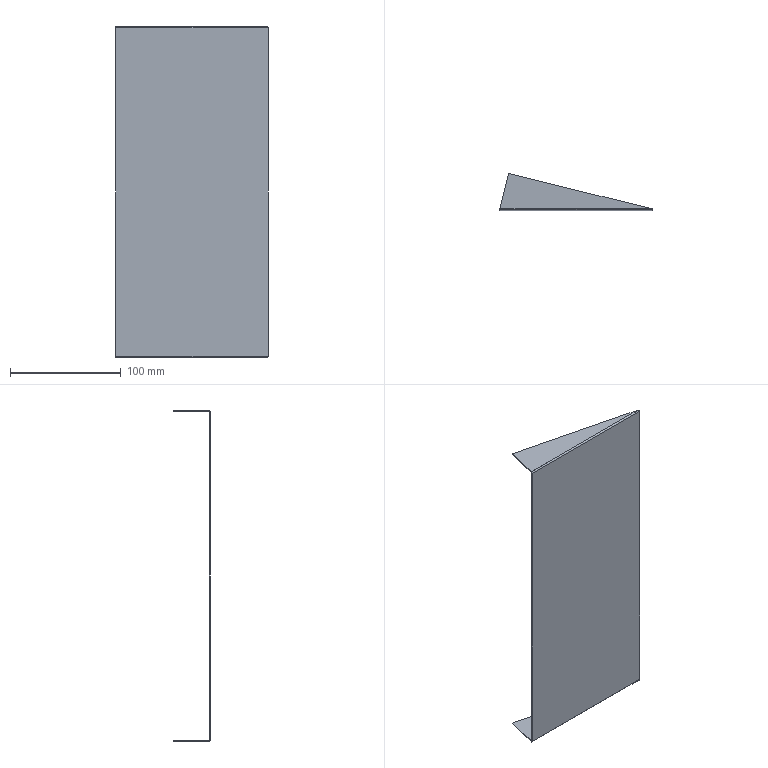Part | SolidWorks | features EdgeFlange 1, FlatPattern 1, MirrorPattern 1, SMBaseFlange 1, SheetMetal 1 | 1 solid | 20 faces | box 137.5 x 33 x 299 mm | volume 45429 mm3 | plane 12 | spline 4 | cylinder 4 | commonest cylinder face diameters 0.4 x2 2.4 x2
STEP:
#1=CARTESIAN_POINT('',(0.,-1.,148.3));
#2=VERTEX_POINT('',#1);
#3=CARTESIAN_POINT('',(-137.5,-1.,148.3));
#4=VERTEX_POINT('',#3);
#5=CARTESIAN_POINT('',(0.,-1.,148.3));
#6=DIRECTION('',(-1.,0.,0.));
#7=VECTOR('',#6,1000.);
#8=LINE('',#5,#7);
#9=EDGE_CURVE('',#2,#4,#8,.T.);
#10=ORIENTED_EDGE('',*,*,#9,.T.);
#11=CARTESIAN_POINT('',(-137.5,-1.,-148.3));
#12=VERTEX_POINT('',#11);
#13=CARTESIAN_POINT('',(-137.5,-1.,149.5));
#14=DIRECTION('',(0.,0.,-1.));
#15=VECTOR('',#14,1000.);
#16=LINE('',#13,#15);
#17=EDGE_CURVE('',#4,#12,#16,.T.);
#18=ORIENTED_EDGE('',*,*,#17,.T.);
#19=CARTESIAN_POINT('',(0.,-1.,-148.3));
#20=VERTEX_POINT('',#19);
#21=CARTESIAN_POINT('',(-137.5,-1.,-148.3));
#22=DIRECTION('',(1.,0.,0.));
#23=VECTOR('',#22,1000.);
#24=LINE('',#21,#23);
#25=EDGE_CURVE('',#12,#20,#24,.T.);
#26=ORIENTED_EDGE('',*,*,#25,.T.);
#27=CARTESIAN_POINT('',(0.,-1.,149.5));
#28=DIRECTION('',(0.,0.,-1.));
#29=VECTOR('',#28,1000.);
#30=LINE('',#27,#29);
#31=EDGE_CURVE('',#2,#20,#30,.T.);
#32=ORIENTED_EDGE('',*,*,#31,.F.);
#33=EDGE_LOOP('',(#10,#18,#26,#32));
#34=FACE_OUTER_BOUND('',#33,.T.);
#35=CARTESIAN_POINT('',(-137.5,-1.,149.5));
#36=DIRECTION('',(0.,1.,0.));
#37=DIRECTION('',(0.,0.,1.));
#38=AXIS2_PLACEMENT_3D('',#35,#36,#37);
#39=PLANE('',#38);
#40=ADVANCED_FACE('',(#34),#39,.F.);
#41=CARTESIAN_POINT('',(-137.5,0.,148.3));
#42=VERTEX_POINT('',#41);
#43=CARTESIAN_POINT('',(-137.5,0.,-148.3));
#44=VERTEX_POINT('',#43);
#45=CARTESIAN_POINT('',(-137.5,0.,149.5));
#46=DIRECTION('',(0.,0.,-1.));
#47=VECTOR('',#46,1000.);
#48=LINE('',#45,#47);
#49=EDGE_CURVE('',#42,#44,#48,.T.);
#50=ORIENTED_EDGE('',*,*,#49,.F.);
#51=CARTESIAN_POINT('',(0.,0.,148.3));
#52=VERTEX_POINT('',#51);
#53=CARTESIAN_POINT('',(0.,0.,148.3));
#54=DIRECTION('',(-1.,0.,0.));
#55=VECTOR('',#54,1000.);
#56=LINE('',#53,#55);
#57=EDGE_CURVE('',#52,#42,#56,.T.);
#58=ORIENTED_EDGE('',*,*,#57,.F.);
#59=CARTESIAN_POINT('',(0.,0.,-148.3));
#60=VERTEX_POINT('',#59);
#61=CARTESIAN_POINT('',(0.,0.,149.5));
#62=DIRECTION('',(0.,0.,-1.));
#63=VECTOR('',#62,1000.);
#64=LINE('',#61,#63);
#65=EDGE_CURVE('',#52,#60,#64,.T.);
#66=ORIENTED_EDGE('',*,*,#65,.T.);
#67=CARTESIAN_POINT('',(-137.5,0.,-148.3));
#68=DIRECTION('',(1.,0.,0.));
#69=VECTOR('',#68,1000.);
#70=LINE('',#67,#69);
#71=EDGE_CURVE('',#44,#60,#70,.T.);
#72=ORIENTED_EDGE('',*,*,#71,.F.);
#73=EDGE_LOOP('',(#50,#58,#66,#72));
#74=FACE_OUTER_BOUND('',#73,.T.);
#75=CARTESIAN_POINT('',(-137.5,0.,149.5));
#76=DIRECTION('',(0.,1.,0.));
#77=DIRECTION('',(0.,0.,1.));
#78=AXIS2_PLACEMENT_3D('',#75,#76,#77);
#79=PLANE('',#78);
#80=ADVANCED_FACE('',(#74),#79,.T.);
#81=ORIENTED_EDGE('',*,*,#65,.F.);
#82=CARTESIAN_POINT('',(0.,0.,148.3));
#83=DIRECTION('',(0.,-1.,0.));
#84=VECTOR('',#83,1000.);
#85=LINE('',#82,#84);
#86=EDGE_CURVE('',#52,#2,#85,.T.);
#87=ORIENTED_EDGE('',*,*,#86,.T.);
#88=ORIENTED_EDGE('',*,*,#31,.T.);
#89=CARTESIAN_POINT('',(0.,0.,-148.3));
#90=DIRECTION('',(0.,-1.,0.));
#91=VECTOR('',#90,1000.);
#92=LINE('',#89,#91);
#93=EDGE_CURVE('',#60,#20,#92,.T.);
#94=ORIENTED_EDGE('',*,*,#93,.F.);
#95=EDGE_LOOP('',(#81,#87,#88,#94));
#96=FACE_OUTER_BOUND('',#95,.T.);
#97=CARTESIAN_POINT('',(0.,0.,149.5));
#98=DIRECTION('',(1.,0.,0.));
#99=DIRECTION('',(0.,0.,-1.));
#100=AXIS2_PLACEMENT_3D('',#97,#98,#99);
#101=PLANE('',#100);
#102=ADVANCED_FACE('',(#96),#101,.T.);
#103=CARTESIAN_POINT('',(-137.5,0.,148.3));
#104=DIRECTION('',(0.,-1.,0.));
#105=VECTOR('',#104,1000.);
#106=LINE('',#103,#105);
#107=EDGE_CURVE('',#42,#4,#106,.T.);
#108=ORIENTED_EDGE('',*,*,#107,.F.);
#109=ORIENTED_EDGE('',*,*,#49,.T.);
#110=CARTESIAN_POINT('',(-137.5,0.,-148.3));
#111=DIRECTION('',(0.,-1.,0.));
#112=VECTOR('',#111,1000.);
#113=LINE('',#110,#112);
#114=EDGE_CURVE('',#44,#12,#113,.T.);
#115=ORIENTED_EDGE('',*,*,#114,.T.);
#116=ORIENTED_EDGE('',*,*,#17,.F.);
#117=EDGE_LOOP('',(#108,#109,#115,#116));
#118=FACE_OUTER_BOUND('',#117,.T.);
#119=CARTESIAN_POINT('',(-137.5,-1.,149.5));
#120=DIRECTION('',(-1.,0.,0.));
#121=DIRECTION('',(0.,0.,1.));
#122=AXIS2_PLACEMENT_3D('',#119,#120,#121);
#123=PLANE('',#122);
#124=ADVANCED_FACE('',(#118),#123,.T.);
#125=CARTESIAN_POINT('',(-0.81,0.2,-148.5));
#126=VERTEX_POINT('',#125);
#127=CARTESIAN_POINT('',(-0.81,0.2,-149.5));
#128=VERTEX_POINT('',#127);
#129=CARTESIAN_POINT('',(-0.81,0.2,-149.5));
#130=DIRECTION('',(0.,0.,-1.));
#131=VECTOR('',#130,1000.);
#132=LINE('',#129,#131);
#133=EDGE_CURVE('',#126,#128,#132,.T.);
#134=ORIENTED_EDGE('',*,*,#133,.F.);
#135=CARTESIAN_POINT('',(0.,0.,-148.3));
#136=CARTESIAN_POINT('',(-0.135,0.,-148.352));
#137=CARTESIAN_POINT('',(-0.27,0.02155,-148.404));
#138=CARTESIAN_POINT('',(-0.54,0.0956,-148.478));
#139=CARTESIAN_POINT('',(-0.675,0.1476,-148.5));
#140=CARTESIAN_POINT('',(-0.81,0.2,-148.5));
#141=B_SPLINE_CURVE_WITH_KNOTS('',3,(#135,#136,#137,#138,#139,#140),.UNSPECIFIED.,.F.,.F.,(4,2,4),(0.,0.5,1.),.UNSPECIFIED.);
#142=EDGE_CURVE('',#60,#126,#141,.T.);
#143=ORIENTED_EDGE('',*,*,#142,.F.);
#144=ORIENTED_EDGE('',*,*,#93,.T.);
#145=CARTESIAN_POINT('',(0.,-1.,-148.3));
#146=CARTESIAN_POINT('',(-0.06814,-1.,-148.459));
#147=CARTESIAN_POINT('',(-0.1341,-0.9695,-148.612));
#148=CARTESIAN_POINT('',(-0.2703,-0.8484,-148.905));
#149=CARTESIAN_POINT('',(-0.3368,-0.7606,-149.036));
#150=CARTESIAN_POINT('',(-0.4727,-0.5372,-149.26));
#151=CARTESIAN_POINT('',(-0.5396,-0.4051,-149.348));
#152=CARTESIAN_POINT('',(-0.675,-0.1141,-149.469));
#153=CARTESIAN_POINT('',(-0.7418,0.04142,-149.5));
#154=CARTESIAN_POINT('',(-0.81,0.2,-149.5));
#155=B_SPLINE_CURVE_WITH_KNOTS('',3,(#145,#146,#147,#148,#149,#150,#151,#152,#153,#154),.UNSPECIFIED.,.F.,.F.,(4,2,2,2,4),(0.,0.0005093,0.001019,0.001528,0.002037),.UNSPECIFIED.);
#156=EDGE_CURVE('',#20,#128,#155,.T.);
#157=ORIENTED_EDGE('',*,*,#156,.T.);
#158=EDGE_LOOP('',(#134,#143,#144,#157));
#159=FACE_OUTER_BOUND('',#158,.T.);
#160=CARTESIAN_POINT('',(0.,-1.01,-148.3));
#161=CARTESIAN_POINT('',(-0.06751,-1.01,-148.458));
#162=CARTESIAN_POINT('',(-0.135,-0.9785,-148.617));
#163=CARTESIAN_POINT('',(-0.27,-0.8573,-148.909));
#164=CARTESIAN_POINT('',(-0.3375,-0.7676,-149.044));
#165=CARTESIAN_POINT('',(-0.4725,-0.5436,-149.268));
#166=CARTESIAN_POINT('',(-0.54,-0.4094,-149.357));
#167=CARTESIAN_POINT('',(-0.675,-0.1167,-149.479));
#168=CARTESIAN_POINT('',(-0.7425,0.04159,-149.51));
#169=CARTESIAN_POINT('',(-0.81,0.2,-149.51));
#170=CARTESIAN_POINT('',(0.,-1.,-148.3));
#171=CARTESIAN_POINT('',(-0.06751,-1.,-148.457));
#172=CARTESIAN_POINT('',(-0.135,-0.9688,-148.614));
#173=CARTESIAN_POINT('',(-0.27,-0.8485,-148.904));
#174=CARTESIAN_POINT('',(-0.3375,-0.7596,-149.037));
#175=CARTESIAN_POINT('',(-0.4725,-0.5375,-149.26));
#176=CARTESIAN_POINT('',(-0.54,-0.4043,-149.349));
#177=CARTESIAN_POINT('',(-0.675,-0.1141,-149.469));
#178=CARTESIAN_POINT('',(-0.7425,0.0429,-149.5));
#179=CARTESIAN_POINT('',(-0.81,0.2,-149.5));
#180=CARTESIAN_POINT('',(0.,0.,-148.3));
#181=CARTESIAN_POINT('',(-0.0675,0.,-148.326));
#182=CARTESIAN_POINT('',(-0.135,0.005205,-148.352));
#183=CARTESIAN_POINT('',(-0.27,0.02524,-148.401));
#184=CARTESIAN_POINT('',(-0.3375,0.04007,-148.423));
#185=CARTESIAN_POINT('',(-0.4725,0.07709,-148.46));
#186=CARTESIAN_POINT('',(-0.54,0.09928,-148.475));
#187=CARTESIAN_POINT('',(-0.675,0.1477,-148.495));
#188=CARTESIAN_POINT('',(-0.7425,0.1738,-148.5));
#189=CARTESIAN_POINT('',(-0.81,0.2,-148.5));
#190=CARTESIAN_POINT('',(0.,0.0101,-148.3));
#191=CARTESIAN_POINT('',(-0.0675,0.0101,-148.325));
#192=CARTESIAN_POINT('',(-0.135,0.01504,-148.35));
#193=CARTESIAN_POINT('',(-0.27,0.03407,-148.396));
#194=CARTESIAN_POINT('',(-0.3375,0.04814,-148.417));
#195=CARTESIAN_POINT('',(-0.4725,0.0833,-148.452));
#196=CARTESIAN_POINT('',(-0.54,0.1044,-148.466));
#197=CARTESIAN_POINT('',(-0.675,0.1503,-148.485));
#198=CARTESIAN_POINT('',(-0.7425,0.1751,-148.49));
#199=CARTESIAN_POINT('',(-0.81,0.2,-148.49));
#200=B_SPLINE_SURFACE_WITH_KNOTS('',1,3,((#160,#161,#162,#163,#164,#165,#166,#167,#168,#169),(#170,#171,#172,#173,#174,#175,#176,#177,#178,#179),(#180,#181,#182,#183,#184,#185,#186,#187,#188,#189),(#190,#191,#192,#193,#194,#195,#196,#197,#198,#199)),.UNSPECIFIED.,.F.,.F.,.F.,(2,1,1,2),(4,2,2,2,4),(-0.01,0.,1.,1.01),(0.,0.25,0.5,0.75,1.),.UNSPECIFIED.);
#201=ADVANCED_FACE('',(#159),#200,.F.);
#202=CARTESIAN_POINT('',(-137.451,0.2,-148.5));
#203=VERTEX_POINT('',#202);
#204=CARTESIAN_POINT('',(-137.451,0.2,-148.5));
#205=CARTESIAN_POINT('',(-137.459,0.1476,-148.5));
#206=CARTESIAN_POINT('',(-137.467,0.0956,-148.478));
#207=CARTESIAN_POINT('',(-137.484,0.02155,-148.404));
#208=CARTESIAN_POINT('',(-137.492,0.,-148.352));
#209=CARTESIAN_POINT('',(-137.5,0.,-148.3));
#210=B_SPLINE_CURVE_WITH_KNOTS('',3,(#204,#205,#206,#207,#208,#209),.UNSPECIFIED.,.F.,.F.,(4,2,4),(0.,0.5,1.),.UNSPECIFIED.);
#211=EDGE_CURVE('',#203,#44,#210,.T.);
#212=ORIENTED_EDGE('',*,*,#211,.F.);
#213=CARTESIAN_POINT('',(-137.451,0.2,-149.5));
#214=VERTEX_POINT('',#213);
#215=CARTESIAN_POINT('',(-137.451,0.2,-148.5));
#216=DIRECTION('',(0.,0.,-1.));
#217=VECTOR('',#216,1000.);
#218=LINE('',#215,#217);
#219=EDGE_CURVE('',#203,#214,#218,.T.);
#220=ORIENTED_EDGE('',*,*,#219,.T.);
#221=CARTESIAN_POINT('',(-137.451,0.2,-149.5));
#222=CARTESIAN_POINT('',(-137.455,0.04292,-149.5));
#223=CARTESIAN_POINT('',(-137.459,-0.1141,-149.469));
#224=CARTESIAN_POINT('',(-137.467,-0.4043,-149.349));
#225=CARTESIAN_POINT('',(-137.471,-0.5375,-149.26));
#226=CARTESIAN_POINT('',(-137.479,-0.7596,-149.037));
#227=CARTESIAN_POINT('',(-137.484,-0.8485,-148.904));
#228=CARTESIAN_POINT('',(-137.492,-0.9688,-148.614));
#229=CARTESIAN_POINT('',(-137.496,-1.,-148.457));
#230=CARTESIAN_POINT('',(-137.5,-1.,-148.3));
#231=B_SPLINE_CURVE_WITH_KNOTS('',3,(#221,#222,#223,#224,#225,#226,#227,#228,#229,#230),.UNSPECIFIED.,.F.,.F.,(4,2,2,2,4),(0.,0.25,0.5,0.75,1.),.UNSPECIFIED.);
#232=EDGE_CURVE('',#214,#12,#231,.T.);
#233=ORIENTED_EDGE('',*,*,#232,.T.);
#234=ORIENTED_EDGE('',*,*,#114,.F.);
#235=EDGE_LOOP('',(#212,#220,#233,#234));
#236=FACE_OUTER_BOUND('',#235,.T.);
#237=CARTESIAN_POINT('',(-137.451,0.2,-149.51));
#238=CARTESIAN_POINT('',(-137.455,0.04158,-149.51));
#239=CARTESIAN_POINT('',(-137.459,-0.1167,-149.479));
#240=CARTESIAN_POINT('',(-137.467,-0.4094,-149.357));
#241=CARTESIAN_POINT('',(-137.471,-0.5436,-149.268));
#242=CARTESIAN_POINT('',(-137.479,-0.7676,-149.044));
#243=CARTESIAN_POINT('',(-137.484,-0.8573,-148.909));
#244=CARTESIAN_POINT('',(-137.492,-0.9785,-148.617));
#245=CARTESIAN_POINT('',(-137.496,-1.01,-148.458));
#246=CARTESIAN_POINT('',(-137.5,-1.01,-148.3));
#247=CARTESIAN_POINT('',(-137.451,0.2,-149.5));
#248=CARTESIAN_POINT('',(-137.455,0.04289,-149.5));
#249=CARTESIAN_POINT('',(-137.459,-0.1141,-149.469));
#250=CARTESIAN_POINT('',(-137.467,-0.4043,-149.349));
#251=CARTESIAN_POINT('',(-137.471,-0.5375,-149.26));
#252=CARTESIAN_POINT('',(-137.479,-0.7596,-149.037));
#253=CARTESIAN_POINT('',(-137.484,-0.8485,-148.904));
#254=CARTESIAN_POINT('',(-137.492,-0.9688,-148.614));
#255=CARTESIAN_POINT('',(-137.496,-1.,-148.457));
#256=CARTESIAN_POINT('',(-137.5,-1.,-148.3));
#257=CARTESIAN_POINT('',(-137.451,0.2,-148.5));
#258=CARTESIAN_POINT('',(-137.455,0.1738,-148.5));
#259=CARTESIAN_POINT('',(-137.459,0.1477,-148.495));
#260=CARTESIAN_POINT('',(-137.467,0.09928,-148.475));
#261=CARTESIAN_POINT('',(-137.471,0.07709,-148.46));
#262=CARTESIAN_POINT('',(-137.479,0.04007,-148.423));
#263=CARTESIAN_POINT('',(-137.484,0.02524,-148.401));
#264=CARTESIAN_POINT('',(-137.492,0.005205,-148.352));
#265=CARTESIAN_POINT('',(-137.496,0.,-148.326));
#266=CARTESIAN_POINT('',(-137.5,0.,-148.3));
#267=CARTESIAN_POINT('',(-137.451,0.2,-148.49));
#268=CARTESIAN_POINT('',(-137.455,0.1751,-148.49));
#269=CARTESIAN_POINT('',(-137.459,0.1503,-148.485));
#270=CARTESIAN_POINT('',(-137.467,0.1044,-148.466));
#271=CARTESIAN_POINT('',(-137.471,0.0833,-148.452));
#272=CARTESIAN_POINT('',(-137.479,0.04814,-148.417));
#273=CARTESIAN_POINT('',(-137.484,0.03407,-148.396));
#274=CARTESIAN_POINT('',(-137.492,0.01504,-148.35));
#275=CARTESIAN_POINT('',(-137.496,0.0101,-148.325));
#276=CARTESIAN_POINT('',(-137.5,0.0101,-148.3));
#277=B_SPLINE_SURFACE_WITH_KNOTS('',1,3,((#237,#238,#239,#240,#241,#242,#243,#244,#245,#246),(#247,#248,#249,#250,#251,#252,#253,#254,#255,#256),(#257,#258,#259,#260,#261,#262,#263,#264,#265,#266),(#267,#268,#269,#270,#271,#272,#273,#274,#275,#276)),.UNSPECIFIED.,.F.,.F.,.F.,(2,1,1,2),(4,2,2,2,4),(-0.01,0.,1.,1.01),(0.,0.25,0.5,0.75,1.),.UNSPECIFIED.);
#278=ADVANCED_FACE('',(#236),#277,.F.);
#279=ORIENTED_EDGE('',*,*,#25,.F.);
#280=ORIENTED_EDGE('',*,*,#232,.F.);
#281=CARTESIAN_POINT('',(0.,0.2,-149.5));
#282=DIRECTION('',(-1.,0.,0.));
#283=VECTOR('',#282,1000.);
#284=LINE('',#281,#283);
#285=EDGE_CURVE('',#128,#214,#284,.T.);
#286=ORIENTED_EDGE('',*,*,#285,.F.);
#287=ORIENTED_EDGE('',*,*,#156,.F.);
#288=EDGE_LOOP('',(#279,#280,#286,#287));
#289=FACE_OUTER_BOUND('',#288,.T.);
#290=CARTESIAN_POINT('',(-137.5,0.2,-148.3));
#291=DIRECTION('',(-1.,0.,0.));
#292=DIRECTION('',(0.,0.,-1.));
#293=AXIS2_PLACEMENT_3D('',#290,#291,#292);
#294=CYLINDRICAL_SURFACE('',#293,1.2);
#295=ADVANCED_FACE('',(#289),#294,.T.);
#296=ORIENTED_EDGE('',*,*,#71,.T.);
#297=ORIENTED_EDGE('',*,*,#142,.T.);
#298=CARTESIAN_POINT('',(-0.81,0.2,-148.5));
#299=DIRECTION('',(-1.,0.,0.));
#300=VECTOR('',#299,1000.);
#301=LINE('',#298,#300);
#302=EDGE_CURVE('',#126,#203,#301,.T.);
#303=ORIENTED_EDGE('',*,*,#302,.T.);
#304=ORIENTED_EDGE('',*,*,#211,.T.);
#305=EDGE_LOOP('',(#296,#297,#303,#304));
#306=FACE_OUTER_BOUND('',#305,.T.);
#307=CARTESIAN_POINT('',(-137.5,0.2,-148.3));
#308=DIRECTION('',(-1.,0.,0.));
#309=DIRECTION('',(0.,0.,-1.));
#310=AXIS2_PLACEMENT_3D('',#307,#308,#309);
#311=CYLINDRICAL_SURFACE('',#310,0.2);
#312=ADVANCED_FACE('',(#306),#311,.F.);
#313=ORIENTED_EDGE('',*,*,#219,.F.);
#314=CARTESIAN_POINT('',(-129.599,32.,-148.5));
#315=VERTEX_POINT('',#314);
#316=CARTESIAN_POINT('',(-129.599,32.,-148.5));
#317=DIRECTION('',(0.2397,0.9708,0.));
#318=VECTOR('',#317,1000.);
#319=LINE('',#316,#318);
#320=EDGE_CURVE('',#203,#315,#319,.T.);
#321=ORIENTED_EDGE('',*,*,#320,.T.);
#322=CARTESIAN_POINT('',(-129.599,32.,-149.5));
#323=VERTEX_POINT('',#322);
#324=CARTESIAN_POINT('',(-129.599,32.,-149.5));
#325=DIRECTION('',(0.,0.,1.));
#326=VECTOR('',#325,1000.);
#327=LINE('',#324,#326);
#328=EDGE_CURVE('',#323,#315,#327,.T.);
#329=ORIENTED_EDGE('',*,*,#328,.F.);
#330=CARTESIAN_POINT('',(-129.599,32.,-149.5));
#331=DIRECTION('',(0.2397,0.9708,0.));
#332=VECTOR('',#331,1000.);
#333=LINE('',#330,#332);
#334=EDGE_CURVE('',#214,#323,#333,.T.);
#335=ORIENTED_EDGE('',*,*,#334,.F.);
#336=EDGE_LOOP('',(#313,#321,#329,#335));
#337=FACE_OUTER_BOUND('',#336,.T.);
#338=CARTESIAN_POINT('',(-129.599,32.,-149.5));
#339=DIRECTION('',(0.9708,-0.2397,0.));
#340=DIRECTION('',(0.2397,0.9708,0.));
#341=AXIS2_PLACEMENT_3D('',#338,#339,#340);
#342=PLANE('',#341);
#343=ADVANCED_FACE('',(#337),#342,.F.);
#344=ORIENTED_EDGE('',*,*,#133,.T.);
#345=CARTESIAN_POINT('',(0.,0.,-149.5));
#346=DIRECTION('',(0.9708,-0.2397,0.));
#347=VECTOR('',#346,1000.);
#348=LINE('',#345,#347);
#349=EDGE_CURVE('',#323,#128,#348,.T.);
#350=ORIENTED_EDGE('',*,*,#349,.F.);
#351=ORIENTED_EDGE('',*,*,#328,.T.);
#352=CARTESIAN_POINT('',(0.,0.,-148.5));
#353=DIRECTION('',(0.9708,-0.2397,0.));
#354=VECTOR('',#353,1000.);
#355=LINE('',#352,#354);
#356=EDGE_CURVE('',#315,#126,#355,.T.);
#357=ORIENTED_EDGE('',*,*,#356,.T.);
#358=EDGE_LOOP('',(#344,#350,#351,#357));
#359=FACE_OUTER_BOUND('',#358,.T.);
#360=CARTESIAN_POINT('',(0.,0.,-149.5));
#361=DIRECTION('',(-0.2397,-0.9708,0.));
#362=DIRECTION('',(0.9708,-0.2397,0.));
#363=AXIS2_PLACEMENT_3D('',#360,#361,#362);
#364=PLANE('',#363);
#365=ADVANCED_FACE('',(#359),#364,.F.);
#366=ORIENTED_EDGE('',*,*,#349,.T.);
#367=ORIENTED_EDGE('',*,*,#285,.T.);
#368=ORIENTED_EDGE('',*,*,#334,.T.);
#369=EDGE_LOOP('',(#366,#367,#368));
#370=FACE_OUTER_BOUND('',#369,.T.);
#371=CARTESIAN_POINT('',(0.,0.,-149.5));
#372=DIRECTION('',(0.,0.,-1.));
#373=DIRECTION('',(0.,1.,0.));
#374=AXIS2_PLACEMENT_3D('',#371,#372,#373);
#375=PLANE('',#374);
#376=ADVANCED_FACE('',(#370),#375,.T.);
#377=ORIENTED_EDGE('',*,*,#302,.F.);
#378=ORIENTED_EDGE('',*,*,#356,.F.);
#379=ORIENTED_EDGE('',*,*,#320,.F.);
#380=EDGE_LOOP('',(#377,#378,#379));
#381=FACE_OUTER_BOUND('',#380,.T.);
#382=CARTESIAN_POINT('',(0.,0.,-148.5));
#383=DIRECTION('',(0.,0.,-1.));
#384=DIRECTION('',(0.,1.,0.));
#385=AXIS2_PLACEMENT_3D('',#382,#383,#384);
#386=PLANE('',#385);
#387=ADVANCED_FACE('',(#381),#386,.F.);
#388=CARTESIAN_POINT('',(-137.451,0.2,148.5));
#389=VERTEX_POINT('',#388);
#390=CARTESIAN_POINT('',(-137.451,0.2,149.5));
#391=VERTEX_POINT('',#390);
#392=CARTESIAN_POINT('',(-137.451,0.2,149.5));
#393=DIRECTION('',(0.,0.,1.));
#394=VECTOR('',#393,1000.);
#395=LINE('',#392,#394);
#396=EDGE_CURVE('',#389,#391,#395,.T.);
#397=ORIENTED_EDGE('',*,*,#396,.F.);
#398=CARTESIAN_POINT('',(-137.5,0.,148.3));
#399=CARTESIAN_POINT('',(-137.492,0.,148.352));
#400=CARTESIAN_POINT('',(-137.484,0.02155,148.404));
#401=CARTESIAN_POINT('',(-137.467,0.0956,148.478));
#402=CARTESIAN_POINT('',(-137.459,0.1476,148.5));
#403=CARTESIAN_POINT('',(-137.451,0.2,148.5));
#404=B_SPLINE_CURVE_WITH_KNOTS('',3,(#398,#399,#400,#401,#402,#403),.UNSPECIFIED.,.F.,.F.,(4,2,4),(0.,0.5,1.),.UNSPECIFIED.);
#405=EDGE_CURVE('',#42,#389,#404,.T.);
#406=ORIENTED_EDGE('',*,*,#405,.F.);
#407=ORIENTED_EDGE('',*,*,#107,.T.);
#408=CARTESIAN_POINT('',(-137.5,-1.,148.3));
#409=CARTESIAN_POINT('',(-137.496,-1.,148.457));
#410=CARTESIAN_POINT('',(-137.492,-0.9688,148.614));
#411=CARTESIAN_POINT('',(-137.484,-0.8485,148.904));
#412=CARTESIAN_POINT('',(-137.479,-0.7596,149.037));
#413=CARTESIAN_POINT('',(-137.471,-0.5375,149.26));
#414=CARTESIAN_POINT('',(-137.467,-0.4043,149.349));
#415=CARTESIAN_POINT('',(-137.459,-0.1141,149.469));
#416=CARTESIAN_POINT('',(-137.455,0.04292,149.5));
#417=CARTESIAN_POINT('',(-137.451,0.2,149.5));
#418=B_SPLINE_CURVE_WITH_KNOTS('',3,(#408,#409,#410,#411,#412,#413,#414,#415,#416,#417),.UNSPECIFIED.,.F.,.F.,(4,2,2,2,4),(0.,0.25,0.5,0.75,1.),.UNSPECIFIED.);
#419=EDGE_CURVE('',#4,#391,#418,.T.);
#420=ORIENTED_EDGE('',*,*,#419,.T.);
#421=EDGE_LOOP('',(#397,#406,#407,#420));
#422=FACE_OUTER_BOUND('',#421,.T.);
#423=CARTESIAN_POINT('',(-137.5,-1.01,148.3));
#424=CARTESIAN_POINT('',(-137.496,-1.01,148.458));
#425=CARTESIAN_POINT('',(-137.492,-0.9785,148.617));
#426=CARTESIAN_POINT('',(-137.484,-0.8573,148.909));
#427=CARTESIAN_POINT('',(-137.479,-0.7676,149.044));
#428=CARTESIAN_POINT('',(-137.471,-0.5436,149.268));
#429=CARTESIAN_POINT('',(-137.467,-0.4094,149.357));
#430=CARTESIAN_POINT('',(-137.459,-0.1167,149.479));
#431=CARTESIAN_POINT('',(-137.455,0.04158,149.51));
#432=CARTESIAN_POINT('',(-137.451,0.2,149.51));
#433=CARTESIAN_POINT('',(-137.5,-1.,148.3));
#434=CARTESIAN_POINT('',(-137.496,-1.,148.457));
#435=CARTESIAN_POINT('',(-137.492,-0.9688,148.614));
#436=CARTESIAN_POINT('',(-137.484,-0.8485,148.904));
#437=CARTESIAN_POINT('',(-137.479,-0.7596,149.037));
#438=CARTESIAN_POINT('',(-137.471,-0.5375,149.26));
#439=CARTESIAN_POINT('',(-137.467,-0.4043,149.349));
#440=CARTESIAN_POINT('',(-137.459,-0.1141,149.469));
#441=CARTESIAN_POINT('',(-137.455,0.04289,149.5));
#442=CARTESIAN_POINT('',(-137.451,0.2,149.5));
#443=CARTESIAN_POINT('',(-137.5,0.,148.3));
#444=CARTESIAN_POINT('',(-137.496,0.,148.326));
#445=CARTESIAN_POINT('',(-137.492,0.005205,148.352));
#446=CARTESIAN_POINT('',(-137.484,0.02524,148.401));
#447=CARTESIAN_POINT('',(-137.479,0.04007,148.423));
#448=CARTESIAN_POINT('',(-137.471,0.07709,148.46));
#449=CARTESIAN_POINT('',(-137.467,0.09928,148.475));
#450=CARTESIAN_POINT('',(-137.459,0.1477,148.495));
#451=CARTESIAN_POINT('',(-137.455,0.1738,148.5));
#452=CARTESIAN_POINT('',(-137.451,0.2,148.5));
#453=CARTESIAN_POINT('',(-137.5,0.0101,148.3));
#454=CARTESIAN_POINT('',(-137.496,0.0101,148.325));
#455=CARTESIAN_POINT('',(-137.492,0.01504,148.35));
#456=CARTESIAN_POINT('',(-137.484,0.03407,148.396));
#457=CARTESIAN_POINT('',(-137.479,0.04814,148.417));
#458=CARTESIAN_POINT('',(-137.471,0.0833,148.452));
#459=CARTESIAN_POINT('',(-137.467,0.1044,148.466));
#460=CARTESIAN_POINT('',(-137.459,0.1503,148.485));
#461=CARTESIAN_POINT('',(-137.455,0.1751,148.49));
#462=CARTESIAN_POINT('',(-137.451,0.2,148.49));
#463=B_SPLINE_SURFACE_WITH_KNOTS('',1,3,((#423,#424,#425,#426,#427,#428,#429,#430,#431,#432),(#433,#434,#435,#436,#437,#438,#439,#440,#441,#442),(#443,#444,#445,#446,#447,#448,#449,#450,#451,#452),(#453,#454,#455,#456,#457,#458,#459,#460,#461,#462)),.UNSPECIFIED.,.F.,.F.,.F.,(2,1,1,2),(4,2,2,2,4),(-0.01,0.,1.,1.01),(0.,0.25,0.5,0.75,1.),.UNSPECIFIED.);
#464=ADVANCED_FACE('',(#422),#463,.F.);
#465=CARTESIAN_POINT('',(-0.81,0.2,148.5));
#466=VERTEX_POINT('',#465);
#467=CARTESIAN_POINT('',(-0.81,0.2,148.5));
#468=CARTESIAN_POINT('',(-0.675,0.1476,148.5));
#469=CARTESIAN_POINT('',(-0.54,0.0956,148.478));
#470=CARTESIAN_POINT('',(-0.27,0.02155,148.404));
#471=CARTESIAN_POINT('',(-0.135,0.,148.352));
#472=CARTESIAN_POINT('',(0.,0.,148.3));
#473=B_SPLINE_CURVE_WITH_KNOTS('',3,(#467,#468,#469,#470,#471,#472),.UNSPECIFIED.,.F.,.F.,(4,2,4),(0.,0.5,1.),.UNSPECIFIED.);
#474=EDGE_CURVE('',#466,#52,#473,.T.);
#475=ORIENTED_EDGE('',*,*,#474,.F.);
#476=CARTESIAN_POINT('',(-0.81,0.2,149.5));
#477=VERTEX_POINT('',#476);
#478=CARTESIAN_POINT('',(-0.81,0.2,148.5));
#479=DIRECTION('',(0.,0.,1.));
#480=VECTOR('',#479,1000.);
#481=LINE('',#478,#480);
#482=EDGE_CURVE('',#466,#477,#481,.T.);
#483=ORIENTED_EDGE('',*,*,#482,.T.);
#484=CARTESIAN_POINT('',(-0.81,0.2,149.5));
#485=CARTESIAN_POINT('',(-0.7418,0.04142,149.5));
#486=CARTESIAN_POINT('',(-0.6759,-0.112,149.47));
#487=CARTESIAN_POINT('',(-0.5397,-0.405,149.348));
#488=CARTESIAN_POINT('',(-0.4731,-0.5363,149.261));
#489=CARTESIAN_POINT('',(-0.3373,-0.76,149.037));
#490=CARTESIAN_POINT('',(-0.2704,-0.8481,148.905));
#491=CARTESIAN_POINT('',(-0.135,-0.9688,148.614));
#492=CARTESIAN_POINT('',(-0.06814,-1.,148.459));
#493=CARTESIAN_POINT('',(0.,-1.,148.3));
#494=B_SPLINE_CURVE_WITH_KNOTS('',3,(#484,#485,#486,#487,#488,#489,#490,#491,#492,#493),.UNSPECIFIED.,.F.,.F.,(4,2,2,2,4),(0.,0.0005093,0.001019,0.001528,0.002037),.UNSPECIFIED.);
#495=EDGE_CURVE('',#477,#2,#494,.T.);
#496=ORIENTED_EDGE('',*,*,#495,.T.);
#497=ORIENTED_EDGE('',*,*,#86,.F.);
#498=EDGE_LOOP('',(#475,#483,#496,#497));
#499=FACE_OUTER_BOUND('',#498,.T.);
#500=CARTESIAN_POINT('',(-0.81,0.2,149.51));
#501=CARTESIAN_POINT('',(-0.7425,0.04159,149.51));
#502=CARTESIAN_POINT('',(-0.675,-0.1167,149.479));
#503=CARTESIAN_POINT('',(-0.54,-0.4094,149.357));
#504=CARTESIAN_POINT('',(-0.4725,-0.5436,149.268));
#505=CARTESIAN_POINT('',(-0.3375,-0.7676,149.044));
#506=CARTESIAN_POINT('',(-0.27,-0.8573,148.909));
#507=CARTESIAN_POINT('',(-0.135,-0.9785,148.617));
#508=CARTESIAN_POINT('',(-0.06751,-1.01,148.458));
#509=CARTESIAN_POINT('',(0.,-1.01,148.3));
#510=CARTESIAN_POINT('',(-0.81,0.2,149.5));
#511=CARTESIAN_POINT('',(-0.7425,0.0429,149.5));
#512=CARTESIAN_POINT('',(-0.675,-0.1141,149.469));
#513=CARTESIAN_POINT('',(-0.54,-0.4043,149.349));
#514=CARTESIAN_POINT('',(-0.4725,-0.5375,149.26));
#515=CARTESIAN_POINT('',(-0.3375,-0.7596,149.037));
#516=CARTESIAN_POINT('',(-0.27,-0.8485,148.904));
#517=CARTESIAN_POINT('',(-0.135,-0.9688,148.614));
#518=CARTESIAN_POINT('',(-0.06751,-1.,148.457));
#519=CARTESIAN_POINT('',(0.,-1.,148.3));
#520=CARTESIAN_POINT('',(-0.81,0.2,148.5));
#521=CARTESIAN_POINT('',(-0.7425,0.1738,148.5));
#522=CARTESIAN_POINT('',(-0.675,0.1477,148.495));
#523=CARTESIAN_POINT('',(-0.54,0.09928,148.475));
#524=CARTESIAN_POINT('',(-0.4725,0.07709,148.46));
#525=CARTESIAN_POINT('',(-0.3375,0.04007,148.423));
#526=CARTESIAN_POINT('',(-0.27,0.02524,148.401));
#527=CARTESIAN_POINT('',(-0.135,0.005205,148.352));
#528=CARTESIAN_POINT('',(-0.0675,0.,148.326));
#529=CARTESIAN_POINT('',(0.,0.,148.3));
#530=CARTESIAN_POINT('',(-0.81,0.2,148.49));
#531=CARTESIAN_POINT('',(-0.7425,0.1751,148.49));
#532=CARTESIAN_POINT('',(-0.675,0.1503,148.485));
#533=CARTESIAN_POINT('',(-0.54,0.1044,148.466));
#534=CARTESIAN_POINT('',(-0.4725,0.0833,148.452));
#535=CARTESIAN_POINT('',(-0.3375,0.04814,148.417));
#536=CARTESIAN_POINT('',(-0.27,0.03407,148.396));
#537=CARTESIAN_POINT('',(-0.135,0.01504,148.35));
#538=CARTESIAN_POINT('',(-0.0675,0.0101,148.325));
#539=CARTESIAN_POINT('',(0.,0.0101,148.3));
#540=B_SPLINE_SURFACE_WITH_KNOTS('',1,3,((#500,#501,#502,#503,#504,#505,#506,#507,#508,#509),(#510,#511,#512,#513,#514,#515,#516,#517,#518,#519),(#520,#521,#522,#523,#524,#525,#526,#527,#528,#529),(#530,#531,#532,#533,#534,#535,#536,#537,#538,#539)),.UNSPECIFIED.,.F.,.F.,.F.,(2,1,1,2),(4,2,2,2,4),(-0.01,0.,1.,1.01),(0.,0.25,0.5,0.75,1.),.UNSPECIFIED.);
#541=ADVANCED_FACE('',(#499),#540,.F.);
#542=ORIENTED_EDGE('',*,*,#9,.F.);
#543=ORIENTED_EDGE('',*,*,#495,.F.);
#544=CARTESIAN_POINT('',(0.,0.2,149.5));
#545=DIRECTION('',(1.,0.,0.));
#546=VECTOR('',#545,1000.);
#547=LINE('',#544,#546);
#548=EDGE_CURVE('',#391,#477,#547,.T.);
#549=ORIENTED_EDGE('',*,*,#548,.F.);
#550=ORIENTED_EDGE('',*,*,#419,.F.);
#551=EDGE_LOOP('',(#542,#543,#549,#550));
#552=FACE_OUTER_BOUND('',#551,.T.);
#553=CARTESIAN_POINT('',(0.,0.2,148.3));
#554=DIRECTION('',(1.,0.,0.));
#555=DIRECTION('',(0.,0.,1.));
#556=AXIS2_PLACEMENT_3D('',#553,#554,#555);
#557=CYLINDRICAL_SURFACE('',#556,1.2);
#558=ADVANCED_FACE('',(#552),#557,.T.);
#559=ORIENTED_EDGE('',*,*,#57,.T.);
#560=ORIENTED_EDGE('',*,*,#405,.T.);
#561=CARTESIAN_POINT('',(-137.451,0.2,148.5));
#562=DIRECTION('',(1.,0.,0.));
#563=VECTOR('',#562,1000.);
#564=LINE('',#561,#563);
#565=EDGE_CURVE('',#389,#466,#564,.T.);
#566=ORIENTED_EDGE('',*,*,#565,.T.);
#567=ORIENTED_EDGE('',*,*,#474,.T.);
#568=EDGE_LOOP('',(#559,#560,#566,#567));
#569=FACE_OUTER_BOUND('',#568,.T.);
#570=CARTESIAN_POINT('',(0.,0.2,148.3));
#571=DIRECTION('',(1.,0.,0.));
#572=DIRECTION('',(0.,0.,1.));
#573=AXIS2_PLACEMENT_3D('',#570,#571,#572);
#574=CYLINDRICAL_SURFACE('',#573,0.2);
#575=ADVANCED_FACE('',(#569),#574,.F.);
#576=CARTESIAN_POINT('',(-129.599,32.,148.5));
#577=VERTEX_POINT('',#576);
#578=CARTESIAN_POINT('',(-129.599,32.,148.5));
#579=DIRECTION('',(0.2397,0.9708,0.));
#580=VECTOR('',#579,1000.);
#581=LINE('',#578,#580);
#582=EDGE_CURVE('',#389,#577,#581,.T.);
#583=ORIENTED_EDGE('',*,*,#582,.F.);
#584=ORIENTED_EDGE('',*,*,#396,.T.);
#585=CARTESIAN_POINT('',(-129.599,32.,149.5));
#586=VERTEX_POINT('',#585);
#587=CARTESIAN_POINT('',(-129.599,32.,149.5));
#588=DIRECTION('',(0.2397,0.9708,0.));
#589=VECTOR('',#588,1000.);
#590=LINE('',#587,#589);
#591=EDGE_CURVE('',#391,#586,#590,.T.);
#592=ORIENTED_EDGE('',*,*,#591,.T.);
#593=CARTESIAN_POINT('',(-129.599,32.,149.5));
#594=DIRECTION('',(0.,0.,-1.));
#595=VECTOR('',#594,1000.);
#596=LINE('',#593,#595);
#597=EDGE_CURVE('',#586,#577,#596,.T.);
#598=ORIENTED_EDGE('',*,*,#597,.T.);
#599=EDGE_LOOP('',(#583,#584,#592,#598));
#600=FACE_OUTER_BOUND('',#599,.T.);
#601=CARTESIAN_POINT('',(-129.599,32.,149.5));
#602=DIRECTION('',(-0.9708,0.2397,0.));
#603=DIRECTION('',(-0.2397,-0.9708,0.));
#604=AXIS2_PLACEMENT_3D('',#601,#602,#603);
#605=PLANE('',#604);
#606=ADVANCED_FACE('',(#600),#605,.T.);
#607=CARTESIAN_POINT('',(0.,0.,149.5));
#608=DIRECTION('',(0.9708,-0.2397,0.));
#609=VECTOR('',#608,1000.);
#610=LINE('',#607,#609);
#611=EDGE_CURVE('',#586,#477,#610,.T.);
#612=ORIENTED_EDGE('',*,*,#611,.T.);
#613=ORIENTED_EDGE('',*,*,#482,.F.);
#614=CARTESIAN_POINT('',(0.,0.,148.5));
#615=DIRECTION('',(0.9708,-0.2397,0.));
#616=VECTOR('',#615,1000.);
#617=LINE('',#614,#616);
#618=EDGE_CURVE('',#577,#466,#617,.T.);
#619=ORIENTED_EDGE('',*,*,#618,.F.);
#620=ORIENTED_EDGE('',*,*,#597,.F.);
#621=EDGE_LOOP('',(#612,#613,#619,#620));
#622=FACE_OUTER_BOUND('',#621,.T.);
#623=CARTESIAN_POINT('',(0.,0.,149.5));
#624=DIRECTION('',(0.2397,0.9708,0.));
#625=DIRECTION('',(-0.9708,0.2397,0.));
#626=AXIS2_PLACEMENT_3D('',#623,#624,#625);
#627=PLANE('',#626);
#628=ADVANCED_FACE('',(#622),#627,.T.);
#629=ORIENTED_EDGE('',*,*,#591,.F.);
#630=ORIENTED_EDGE('',*,*,#548,.T.);
#631=ORIENTED_EDGE('',*,*,#611,.F.);
#632=EDGE_LOOP('',(#629,#630,#631));
#633=FACE_OUTER_BOUND('',#632,.T.);
#634=CARTESIAN_POINT('',(0.,0.,149.5));
#635=DIRECTION('',(0.,0.,1.));
#636=DIRECTION('',(0.,1.,0.));
#637=AXIS2_PLACEMENT_3D('',#634,#635,#636);
#638=PLANE('',#637);
#639=ADVANCED_FACE('',(#633),#638,.T.);
#640=ORIENTED_EDGE('',*,*,#565,.F.);
#641=ORIENTED_EDGE('',*,*,#582,.T.);
#642=ORIENTED_EDGE('',*,*,#618,.T.);
#643=EDGE_LOOP('',(#640,#641,#642));
#644=FACE_OUTER_BOUND('',#643,.T.);
#645=CARTESIAN_POINT('',(0.,0.,148.5));
#646=DIRECTION('',(0.,0.,1.));
#647=DIRECTION('',(0.,1.,0.));
#648=AXIS2_PLACEMENT_3D('',#645,#646,#647);
#649=PLANE('',#648);
#650=ADVANCED_FACE('',(#644),#649,.F.);
#651=CLOSED_SHELL('',(#40,#80,#102,#124,#201,#278,#295,#312,#343,#365,#376,#387,#464,#541,#558,#575,#606,#628,#639,#650));
#652=MANIFOLD_SOLID_BREP('',#651);
#653=CARTESIAN_POINT('',(0.,0.,0.));
#654=DIRECTION('',(0.,0.,1.));
#655=DIRECTION('',(1.,0.,0.));
#656=AXIS2_PLACEMENT_3D('',#653,#654,#655);
#657=(LENGTH_UNIT()NAMED_UNIT(*)SI_UNIT(.MILLI.,.METRE.));
#658=UNCERTAINTY_MEASURE_WITH_UNIT(LENGTH_MEASURE(0.00001),#657,'','');
#659=(NAMED_UNIT(*)PLANE_ANGLE_UNIT()SI_UNIT($,.RADIAN.));
#660=(NAMED_UNIT(*)SI_UNIT($,.STERADIAN.)SOLID_ANGLE_UNIT());
#661=(GEOMETRIC_REPRESENTATION_CONTEXT(3)GLOBAL_UNCERTAINTY_ASSIGNED_CONTEXT((#658))GLOBAL_UNIT_ASSIGNED_CONTEXT((#657,#659,#660))REPRESENTATION_CONTEXT('',''));
#662=ADVANCED_BREP_SHAPE_REPRESENTATION('',(#652,#656),#661);